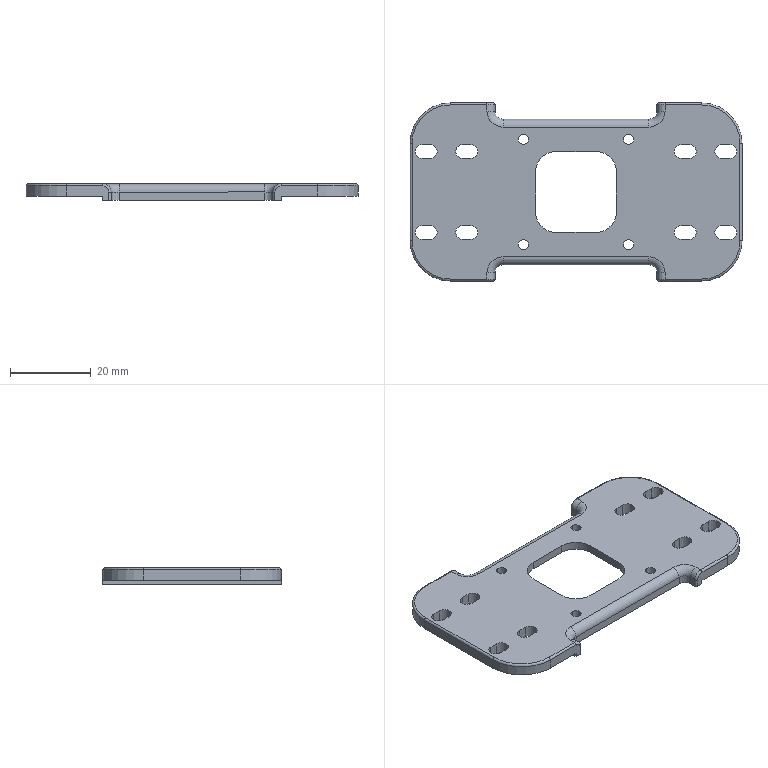Part | 1 solid | 133 faces | box 82 x 44 x 4 mm | volume 7655 mm3 | cylinder 78 | plane 43 | torus 12 | commonest cylinder face diameters 4 x24 3.4 x16 6.2 x12 1 x10 2.5 x8 10 x4